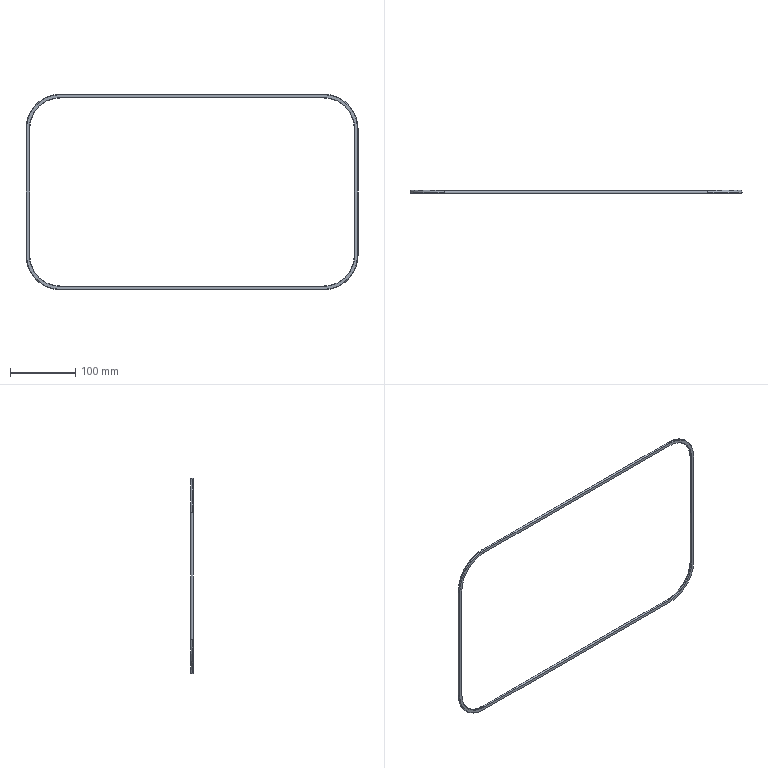Part | STEP file | P-0102091 | 1 solid | 17 faces | box 508.6 x 4.6 x 299.7 mm | volume 33274 mm3 | torus 12 | cylinder 4 | plane 1 | commonest cylinder face diameters 5.7 x4
STEP:
#1=CARTESIAN_POINT('',(0.,0.,0.));
#2=DIRECTION('',(0.,0.,1.));
#3=DIRECTION('',(1.,0.,0.));
#4=AXIS2_PLACEMENT_3D('',#1,#2,#3);
#5=CARTESIAN_POINT('',(-248.8,0.,-91.5));
#6=VERTEX_POINT('',#5);
#7=CARTESIAN_POINT('',(-248.199,-1.75,-91.5));
#8=VERTEX_POINT('',#7);
#9=CARTESIAN_POINT('',(-245.95,0.,-91.5));
#10=DIRECTION('',(0.,0.,1.));
#11=DIRECTION('',(0.,-1.,0.));
#12=AXIS2_PLACEMENT_3D('',#9,#10,#11);
#13=CIRCLE('',#12,2.85);
#14=CARTESIAN_POINT('',(-195.95,0.,-91.5));
#15=DIRECTION('',(0.,-1.,0.));
#16=DIRECTION('',(0.,0.,-1.));
#17=AXIS2_PLACEMENT_3D('',#14,#15,#16);
#18=TOROIDAL_SURFACE('',#17,50.,2.85);
#19=CARTESIAN_POINT('',(4.712,-4.712));
#20=DIRECTION('',(0.,1.));
#21=VECTOR('',#20,1.);
#22=LINE('',#19,#21);
#23=(GEOMETRIC_REPRESENTATION_CONTEXT(2)PARAMETRIC_REPRESENTATION_CONTEXT()REPRESENTATION_CONTEXT('',''));
#24=DEFINITIONAL_REPRESENTATION('',(#22),#23);
#25=PCURVE('',#18,#24);
#26=CARTESIAN_POINT('',(-245.95,0.,102.5));
#27=DIRECTION('',(0.,0.,-1.));
#28=DIRECTION('',(0.,-1.,0.));
#29=AXIS2_PLACEMENT_3D('',#26,#27,#28);
#30=CYLINDRICAL_SURFACE('',#29,2.85);
#31=CARTESIAN_POINT('',(6.283,194.));
#32=DIRECTION('',(-1.,0.));
#33=VECTOR('',#32,1.);
#34=LINE('',#31,#33);
#35=(GEOMETRIC_REPRESENTATION_CONTEXT(2)PARAMETRIC_REPRESENTATION_CONTEXT()REPRESENTATION_CONTEXT('',''));
#36=DEFINITIONAL_REPRESENTATION('',(#34),#35);
#37=PCURVE('',#30,#36);
#38=SURFACE_CURVE('',#13,(#25,#37),.PCURVE_S1.);
#39=EDGE_CURVE('',#6,#8,#38,.T.);
#40=ORIENTED_EDGE('',*,*,#39,.F.);
#41=CARTESIAN_POINT('',(-195.95,0.,-144.35));
#42=VERTEX_POINT('',#41);
#43=CARTESIAN_POINT('',(-195.95,0.,-91.5));
#44=DIRECTION('',(0.,-1.,0.));
#45=DIRECTION('',(1.,0.,0.));
#46=AXIS2_PLACEMENT_3D('',#43,#44,#45);
#47=CIRCLE('',#46,52.85);
#48=CARTESIAN_POINT('',(1.571,0.));
#49=DIRECTION('',(1.,0.));
#50=VECTOR('',#49,1.);
#51=LINE('',#48,#50);
#52=(GEOMETRIC_REPRESENTATION_CONTEXT(2)PARAMETRIC_REPRESENTATION_CONTEXT()REPRESENTATION_CONTEXT('',''));
#53=DEFINITIONAL_REPRESENTATION('',(#51),#52);
#54=PCURVE('',#18,#53);
#55=CARTESIAN_POINT('',(-195.95,0.,-91.5));
#56=DIRECTION('',(0.,-1.,0.));
#57=DIRECTION('',(0.,0.,-1.));
#58=AXIS2_PLACEMENT_3D('',#55,#56,#57);
#59=TOROIDAL_SURFACE('',#58,50.,2.85);
#60=CARTESIAN_POINT('',(1.571,6.283));
#61=DIRECTION('',(1.,0.));
#62=VECTOR('',#61,1.);
#63=LINE('',#60,#62);
#64=(GEOMETRIC_REPRESENTATION_CONTEXT(2)PARAMETRIC_REPRESENTATION_CONTEXT()REPRESENTATION_CONTEXT('',''));
#65=DEFINITIONAL_REPRESENTATION('',(#63),#64);
#66=PCURVE('',#59,#65);
#67=SURFACE_CURVE('',#47,(#54,#66),.PCURVE_S1.);
#68=EDGE_CURVE('',#6,#42,#67,.T.);
#69=ORIENTED_EDGE('',*,*,#68,.T.);
#70=CARTESIAN_POINT('',(-195.95,-1.75,-143.749));
#71=VERTEX_POINT('',#70);
#72=CARTESIAN_POINT('',(-195.95,0.,-141.5));
#73=DIRECTION('',(-1.,0.,0.));
#74=DIRECTION('',(0.,-1.,0.));
#75=AXIS2_PLACEMENT_3D('',#72,#73,#74);
#76=CIRCLE('',#75,2.85);
#77=CARTESIAN_POINT('',(6.283,-4.712));
#78=DIRECTION('',(0.,1.));
#79=VECTOR('',#78,1.);
#80=LINE('',#77,#79);
#81=(GEOMETRIC_REPRESENTATION_CONTEXT(2)PARAMETRIC_REPRESENTATION_CONTEXT()REPRESENTATION_CONTEXT('',''));
#82=DEFINITIONAL_REPRESENTATION('',(#80),#81);
#83=PCURVE('',#18,#82);
#84=CARTESIAN_POINT('',(-195.95,0.,-141.5));
#85=DIRECTION('',(1.,0.,0.));
#86=DIRECTION('',(0.,-1.,0.));
#87=AXIS2_PLACEMENT_3D('',#84,#85,#86);
#88=CYLINDRICAL_SURFACE('',#87,2.85);
#89=CARTESIAN_POINT('',(6.283,0.));
#90=DIRECTION('',(-1.,0.));
#91=VECTOR('',#90,1.);
#92=LINE('',#89,#91);
#93=(GEOMETRIC_REPRESENTATION_CONTEXT(2)PARAMETRIC_REPRESENTATION_CONTEXT()REPRESENTATION_CONTEXT('',''));
#94=DEFINITIONAL_REPRESENTATION('',(#92),#93);
#95=PCURVE('',#88,#94);
#96=SURFACE_CURVE('',#76,(#83,#95),.PCURVE_S1.);
#97=EDGE_CURVE('',#42,#71,#96,.T.);
#98=ORIENTED_EDGE('',*,*,#97,.T.);
#99=CARTESIAN_POINT('',(-195.95,-1.75,-91.5));
#100=DIRECTION('',(0.,1.,0.));
#101=DIRECTION('',(0.,0.,-1.));
#102=AXIS2_PLACEMENT_3D('',#99,#100,#101);
#103=CIRCLE('',#102,52.249);
#104=CARTESIAN_POINT('',(6.283,0.6612));
#105=DIRECTION('',(-1.,0.));
#106=VECTOR('',#105,1.);
#107=LINE('',#104,#106);
#108=(GEOMETRIC_REPRESENTATION_CONTEXT(2)PARAMETRIC_REPRESENTATION_CONTEXT()REPRESENTATION_CONTEXT('',''));
#109=DEFINITIONAL_REPRESENTATION('',(#107),#108);
#110=PCURVE('',#18,#109);
#111=CARTESIAN_POINT('',(-195.95,-1.75,158.523));
#112=DIRECTION('',(0.,1.,0.));
#113=DIRECTION('',(1.,0.,0.));
#114=AXIS2_PLACEMENT_3D('',#111,#112,#113);
#115=PLANE('',#114);
#116=CARTESIAN_POINT('',(0.,250.023));
#117=DIRECTION('',(0.,1.));
#118=AXIS2_PLACEMENT_2D('',#116,#117);
#119=CIRCLE('',#118,52.249);
#120=(GEOMETRIC_REPRESENTATION_CONTEXT(2)PARAMETRIC_REPRESENTATION_CONTEXT()REPRESENTATION_CONTEXT('',''));
#121=DEFINITIONAL_REPRESENTATION('',(#119),#120);
#122=PCURVE('',#115,#121);
#123=SURFACE_CURVE('',#103,(#110,#122),.PCURVE_S1.);
#124=EDGE_CURVE('',#71,#8,#123,.T.);
#125=ORIENTED_EDGE('',*,*,#124,.T.);
#126=EDGE_LOOP('',(#40,#69,#98,#125));
#127=FACE_BOUND('',#126,.T.);
#128=ADVANCED_FACE('',(#127),#18,.T.);
#129=ORIENTED_EDGE('',*,*,#68,.F.);
#130=CARTESIAN_POINT('',(-243.1,0.,-91.5));
#131=VERTEX_POINT('',#130);
#132=CARTESIAN_POINT('',(-245.95,0.,-91.5));
#133=DIRECTION('',(0.,0.,1.));
#134=DIRECTION('',(0.,-1.,0.));
#135=AXIS2_PLACEMENT_3D('',#132,#133,#134);
#136=CIRCLE('',#135,2.85);
#137=CARTESIAN_POINT('',(4.712,1.571));
#138=DIRECTION('',(0.,1.));
#139=VECTOR('',#138,1.);
#140=LINE('',#137,#139);
#141=(GEOMETRIC_REPRESENTATION_CONTEXT(2)PARAMETRIC_REPRESENTATION_CONTEXT()REPRESENTATION_CONTEXT('',''));
#142=DEFINITIONAL_REPRESENTATION('',(#140),#141);
#143=PCURVE('',#59,#142);
#144=CARTESIAN_POINT('',(6.283,194.));
#145=DIRECTION('',(-1.,0.));
#146=VECTOR('',#145,1.);
#147=LINE('',#144,#146);
#148=(GEOMETRIC_REPRESENTATION_CONTEXT(2)PARAMETRIC_REPRESENTATION_CONTEXT()REPRESENTATION_CONTEXT('',''));
#149=DEFINITIONAL_REPRESENTATION('',(#147),#148);
#150=PCURVE('',#30,#149);
#151=SURFACE_CURVE('',#136,(#143,#150),.PCURVE_S1.);
#152=EDGE_CURVE('',#131,#6,#151,.T.);
#153=ORIENTED_EDGE('',*,*,#152,.F.);
#154=CARTESIAN_POINT('',(-195.95,0.,-138.65));
#155=VERTEX_POINT('',#154);
#156=CARTESIAN_POINT('',(-195.95,0.,-91.5));
#157=DIRECTION('',(0.,-1.,0.));
#158=DIRECTION('',(1.,0.,0.));
#159=AXIS2_PLACEMENT_3D('',#156,#157,#158);
#160=CIRCLE('',#159,47.15);
#161=CARTESIAN_POINT('',(1.571,3.142));
#162=DIRECTION('',(1.,0.));
#163=VECTOR('',#162,1.);
#164=LINE('',#161,#163);
#165=(GEOMETRIC_REPRESENTATION_CONTEXT(2)PARAMETRIC_REPRESENTATION_CONTEXT()REPRESENTATION_CONTEXT('',''));
#166=DEFINITIONAL_REPRESENTATION('',(#164),#165);
#167=PCURVE('',#59,#166);
#168=CARTESIAN_POINT('',(-195.95,0.,-91.5));
#169=DIRECTION('',(0.,-1.,0.));
#170=DIRECTION('',(0.,0.,-1.));
#171=AXIS2_PLACEMENT_3D('',#168,#169,#170);
#172=TOROIDAL_SURFACE('',#171,50.,2.85);
#173=CARTESIAN_POINT('',(1.571,3.142));
#174=DIRECTION('',(1.,0.));
#175=VECTOR('',#174,1.);
#176=LINE('',#173,#175);
#177=(GEOMETRIC_REPRESENTATION_CONTEXT(2)PARAMETRIC_REPRESENTATION_CONTEXT()REPRESENTATION_CONTEXT('',''));
#178=DEFINITIONAL_REPRESENTATION('',(#176),#177);
#179=PCURVE('',#172,#178);
#180=SURFACE_CURVE('',#160,(#167,#179),.PCURVE_S1.);
#181=EDGE_CURVE('',#131,#155,#180,.T.);
#182=ORIENTED_EDGE('',*,*,#181,.T.);
#183=CARTESIAN_POINT('',(-195.95,0.,-141.5));
#184=DIRECTION('',(-1.,0.,0.));
#185=DIRECTION('',(0.,-1.,0.));
#186=AXIS2_PLACEMENT_3D('',#183,#184,#185);
#187=CIRCLE('',#186,2.85);
#188=CARTESIAN_POINT('',(6.283,1.571));
#189=DIRECTION('',(0.,1.));
#190=VECTOR('',#189,1.);
#191=LINE('',#188,#190);
#192=(GEOMETRIC_REPRESENTATION_CONTEXT(2)PARAMETRIC_REPRESENTATION_CONTEXT()REPRESENTATION_CONTEXT('',''));
#193=DEFINITIONAL_REPRESENTATION('',(#191),#192);
#194=PCURVE('',#59,#193);
#195=CARTESIAN_POINT('',(6.283,0.));
#196=DIRECTION('',(-1.,0.));
#197=VECTOR('',#196,1.);
#198=LINE('',#195,#197);
#199=(GEOMETRIC_REPRESENTATION_CONTEXT(2)PARAMETRIC_REPRESENTATION_CONTEXT()REPRESENTATION_CONTEXT('',''));
#200=DEFINITIONAL_REPRESENTATION('',(#198),#199);
#201=PCURVE('',#88,#200);
#202=SURFACE_CURVE('',#187,(#194,#201),.PCURVE_S1.);
#203=EDGE_CURVE('',#155,#42,#202,.T.);
#204=ORIENTED_EDGE('',*,*,#203,.T.);
#205=EDGE_LOOP('',(#129,#153,#182,#204));
#206=FACE_BOUND('',#205,.T.);
#207=ADVANCED_FACE('',(#206),#59,.T.);
#208=CARTESIAN_POINT('',(-195.95,0.,155.35));
#209=VERTEX_POINT('',#208);
#210=CARTESIAN_POINT('',(-195.95,-1.75,154.749));
#211=VERTEX_POINT('',#210);
#212=CARTESIAN_POINT('',(-195.95,0.,152.5));
#213=DIRECTION('',(1.,0.,0.));
#214=DIRECTION('',(0.,-1.,0.));
#215=AXIS2_PLACEMENT_3D('',#212,#213,#214);
#216=CIRCLE('',#215,2.85);
#217=CARTESIAN_POINT('',(-195.95,0.,102.5));
#218=DIRECTION('',(0.,-1.,0.));
#219=DIRECTION('',(0.,0.,-1.));
#220=AXIS2_PLACEMENT_3D('',#217,#218,#219);
#221=TOROIDAL_SURFACE('',#220,50.,2.85);
#222=CARTESIAN_POINT('',(3.142,-4.712));
#223=DIRECTION('',(0.,1.));
#224=VECTOR('',#223,1.);
#225=LINE('',#222,#224);
#226=(GEOMETRIC_REPRESENTATION_CONTEXT(2)PARAMETRIC_REPRESENTATION_CONTEXT()REPRESENTATION_CONTEXT('',''));
#227=DEFINITIONAL_REPRESENTATION('',(#225),#226);
#228=PCURVE('',#221,#227);
#229=CARTESIAN_POINT('',(206.95,0.,152.5));
#230=DIRECTION('',(-1.,0.,0.));
#231=DIRECTION('',(0.,-1.,0.));
#232=AXIS2_PLACEMENT_3D('',#229,#230,#231);
#233=CYLINDRICAL_SURFACE('',#232,2.85);
#234=CARTESIAN_POINT('',(6.283,402.9));
#235=DIRECTION('',(-1.,0.));
#236=VECTOR('',#235,1.);
#237=LINE('',#234,#236);
#238=(GEOMETRIC_REPRESENTATION_CONTEXT(2)PARAMETRIC_REPRESENTATION_CONTEXT()REPRESENTATION_CONTEXT('',''));
#239=DEFINITIONAL_REPRESENTATION('',(#237),#238);
#240=PCURVE('',#233,#239);
#241=SURFACE_CURVE('',#216,(#228,#240),.PCURVE_S1.);
#242=EDGE_CURVE('',#209,#211,#241,.T.);
#243=ORIENTED_EDGE('',*,*,#242,.F.);
#244=CARTESIAN_POINT('',(-248.8,0.,102.5));
#245=VERTEX_POINT('',#244);
#246=CARTESIAN_POINT('',(-195.95,0.,102.5));
#247=DIRECTION('',(0.,-1.,0.));
#248=DIRECTION('',(1.,0.,0.));
#249=AXIS2_PLACEMENT_3D('',#246,#247,#248);
#250=CIRCLE('',#249,52.85);
#251=CARTESIAN_POINT('',(1.571,0.));
#252=DIRECTION('',(1.,0.));
#253=VECTOR('',#252,1.);
#254=LINE('',#251,#253);
#255=(GEOMETRIC_REPRESENTATION_CONTEXT(2)PARAMETRIC_REPRESENTATION_CONTEXT()REPRESENTATION_CONTEXT('',''));
#256=DEFINITIONAL_REPRESENTATION('',(#254),#255);
#257=PCURVE('',#221,#256);
#258=CARTESIAN_POINT('',(-195.95,0.,102.5));
#259=DIRECTION('',(0.,-1.,0.));
#260=DIRECTION('',(0.,0.,-1.));
#261=AXIS2_PLACEMENT_3D('',#258,#259,#260);
#262=TOROIDAL_SURFACE('',#261,50.,2.85);
#263=CARTESIAN_POINT('',(1.571,6.283));
#264=DIRECTION('',(1.,0.));
#265=VECTOR('',#264,1.);
#266=LINE('',#263,#265);
#267=(GEOMETRIC_REPRESENTATION_CONTEXT(2)PARAMETRIC_REPRESENTATION_CONTEXT()REPRESENTATION_CONTEXT('',''));
#268=DEFINITIONAL_REPRESENTATION('',(#266),#267);
#269=PCURVE('',#262,#268);
#270=SURFACE_CURVE('',#250,(#257,#269),.PCURVE_S1.);
#271=EDGE_CURVE('',#209,#245,#270,.T.);
#272=ORIENTED_EDGE('',*,*,#271,.T.);
#273=CARTESIAN_POINT('',(-248.199,-1.75,102.5));
#274=VERTEX_POINT('',#273);
#275=CARTESIAN_POINT('',(-245.95,0.,102.5));
#276=DIRECTION('',(0.,0.,1.));
#277=DIRECTION('',(0.,-1.,0.));
#278=AXIS2_PLACEMENT_3D('',#275,#276,#277);
#279=CIRCLE('',#278,2.85);
#280=CARTESIAN_POINT('',(4.712,-4.712));
#281=DIRECTION('',(0.,1.));
#282=VECTOR('',#281,1.);
#283=LINE('',#280,#282);
#284=(GEOMETRIC_REPRESENTATION_CONTEXT(2)PARAMETRIC_REPRESENTATION_CONTEXT()REPRESENTATION_CONTEXT('',''));
#285=DEFINITIONAL_REPRESENTATION('',(#283),#284);
#286=PCURVE('',#221,#285);
#287=CARTESIAN_POINT('',(6.283,0.));
#288=DIRECTION('',(-1.,0.));
#289=VECTOR('',#288,1.);
#290=LINE('',#287,#289);
#291=(GEOMETRIC_REPRESENTATION_CONTEXT(2)PARAMETRIC_REPRESENTATION_CONTEXT()REPRESENTATION_CONTEXT('',''));
#292=DEFINITIONAL_REPRESENTATION('',(#290),#291);
#293=PCURVE('',#30,#292);
#294=SURFACE_CURVE('',#279,(#286,#293),.PCURVE_S1.);
#295=EDGE_CURVE('',#245,#274,#294,.T.);
#296=ORIENTED_EDGE('',*,*,#295,.T.);
#297=CARTESIAN_POINT('',(-195.95,-1.75,102.5));
#298=DIRECTION('',(0.,1.,0.));
#299=DIRECTION('',(0.,0.,-1.));
#300=AXIS2_PLACEMENT_3D('',#297,#298,#299);
#301=CIRCLE('',#300,52.249);
#302=CARTESIAN_POINT('',(6.283,0.6612));
#303=DIRECTION('',(-1.,0.));
#304=VECTOR('',#303,1.);
#305=LINE('',#302,#304);
#306=(GEOMETRIC_REPRESENTATION_CONTEXT(2)PARAMETRIC_REPRESENTATION_CONTEXT()REPRESENTATION_CONTEXT('',''));
#307=DEFINITIONAL_REPRESENTATION('',(#305),#306);
#308=PCURVE('',#221,#307);
#309=CARTESIAN_POINT('',(0.,56.023));
#310=DIRECTION('',(0.,1.));
#311=AXIS2_PLACEMENT_2D('',#309,#310);
#312=CIRCLE('',#311,52.249);
#313=(GEOMETRIC_REPRESENTATION_CONTEXT(2)PARAMETRIC_REPRESENTATION_CONTEXT()REPRESENTATION_CONTEXT('',''));
#314=DEFINITIONAL_REPRESENTATION('',(#312),#313);
#315=PCURVE('',#115,#314);
#316=SURFACE_CURVE('',#301,(#308,#315),.PCURVE_S1.);
#317=EDGE_CURVE('',#274,#211,#316,.T.);
#318=ORIENTED_EDGE('',*,*,#317,.T.);
#319=EDGE_LOOP('',(#243,#272,#296,#318));
#320=FACE_BOUND('',#319,.T.);
#321=ADVANCED_FACE('',(#320),#221,.T.);
#322=ORIENTED_EDGE('',*,*,#271,.F.);
#323=CARTESIAN_POINT('',(-195.95,0.,149.65));
#324=VERTEX_POINT('',#323);
#325=CARTESIAN_POINT('',(-195.95,0.,152.5));
#326=DIRECTION('',(1.,0.,0.));
#327=DIRECTION('',(0.,-1.,0.));
#328=AXIS2_PLACEMENT_3D('',#325,#326,#327);
#329=CIRCLE('',#328,2.85);
#330=CARTESIAN_POINT('',(3.142,1.571));
#331=DIRECTION('',(0.,1.));
#332=VECTOR('',#331,1.);
#333=LINE('',#330,#332);
#334=(GEOMETRIC_REPRESENTATION_CONTEXT(2)PARAMETRIC_REPRESENTATION_CONTEXT()REPRESENTATION_CONTEXT('',''));
#335=DEFINITIONAL_REPRESENTATION('',(#333),#334);
#336=PCURVE('',#262,#335);
#337=CARTESIAN_POINT('',(6.283,402.9));
#338=DIRECTION('',(-1.,0.));
#339=VECTOR('',#338,1.);
#340=LINE('',#337,#339);
#341=(GEOMETRIC_REPRESENTATION_CONTEXT(2)PARAMETRIC_REPRESENTATION_CONTEXT()REPRESENTATION_CONTEXT('',''));
#342=DEFINITIONAL_REPRESENTATION('',(#340),#341);
#343=PCURVE('',#233,#342);
#344=SURFACE_CURVE('',#329,(#336,#343),.PCURVE_S1.);
#345=EDGE_CURVE('',#324,#209,#344,.T.);
#346=ORIENTED_EDGE('',*,*,#345,.F.);
#347=CARTESIAN_POINT('',(-243.1,0.,102.5));
#348=VERTEX_POINT('',#347);
#349=CARTESIAN_POINT('',(-195.95,0.,102.5));
#350=DIRECTION('',(0.,-1.,0.));
#351=DIRECTION('',(1.,0.,0.));
#352=AXIS2_PLACEMENT_3D('',#349,#350,#351);
#353=CIRCLE('',#352,47.15);
#354=CARTESIAN_POINT('',(1.571,3.142));
#355=DIRECTION('',(1.,0.));
#356=VECTOR('',#355,1.);
#357=LINE('',#354,#356);
#358=(GEOMETRIC_REPRESENTATION_CONTEXT(2)PARAMETRIC_REPRESENTATION_CONTEXT()REPRESENTATION_CONTEXT('',''));
#359=DEFINITIONAL_REPRESENTATION('',(#357),#358);
#360=PCURVE('',#262,#359);
#361=CARTESIAN_POINT('',(-195.95,0.,102.5));
#362=DIRECTION('',(0.,-1.,0.));
#363=DIRECTION('',(0.,0.,-1.));
#364=AXIS2_PLACEMENT_3D('',#361,#362,#363);
#365=TOROIDAL_SURFACE('',#364,50.,2.85);
#366=CARTESIAN_POINT('',(1.571,3.142));
#367=DIRECTION('',(1.,0.));
#368=VECTOR('',#367,1.);
#369=LINE('',#366,#368);
#370=(GEOMETRIC_REPRESENTATION_CONTEXT(2)PARAMETRIC_REPRESENTATION_CONTEXT()REPRESENTATION_CONTEXT('',''));
#371=DEFINITIONAL_REPRESENTATION('',(#369),#370);
#372=PCURVE('',#365,#371);
#373=SURFACE_CURVE('',#353,(#360,#372),.PCURVE_S1.);
#374=EDGE_CURVE('',#324,#348,#373,.T.);
#375=ORIENTED_EDGE('',*,*,#374,.T.);
#376=CARTESIAN_POINT('',(-245.95,0.,102.5));
#377=DIRECTION('',(0.,0.,1.));
#378=DIRECTION('',(0.,-1.,0.));
#379=AXIS2_PLACEMENT_3D('',#376,#377,#378);
#380=CIRCLE('',#379,2.85);
#381=CARTESIAN_POINT('',(4.712,1.571));
#382=DIRECTION('',(0.,1.));
#383=VECTOR('',#382,1.);
#384=LINE('',#381,#383);
#385=(GEOMETRIC_REPRESENTATION_CONTEXT(2)PARAMETRIC_REPRESENTATION_CONTEXT()REPRESENTATION_CONTEXT('',''));
#386=DEFINITIONAL_REPRESENTATION('',(#384),#385);
#387=PCURVE('',#262,#386);
#388=CARTESIAN_POINT('',(6.283,0.));
#389=DIRECTION('',(-1.,0.));
#390=VECTOR('',#389,1.);
#391=LINE('',#388,#390);
#392=(GEOMETRIC_REPRESENTATION_CONTEXT(2)PARAMETRIC_REPRESENTATION_CONTEXT()REPRESENTATION_CONTEXT('',''));
#393=DEFINITIONAL_REPRESENTATION('',(#391),#392);
#394=PCURVE('',#30,#393);
#395=SURFACE_CURVE('',#380,(#387,#394),.PCURVE_S1.);
#396=EDGE_CURVE('',#348,#245,#395,.T.);
#397=ORIENTED_EDGE('',*,*,#396,.T.);
#398=EDGE_LOOP('',(#322,#346,#375,#397));
#399=FACE_BOUND('',#398,.T.);
#400=ADVANCED_FACE('',(#399),#262,.T.);
#401=CARTESIAN_POINT('',(259.8,0.,102.5));
#402=VERTEX_POINT('',#401);
#403=CARTESIAN_POINT('',(259.199,-1.75,102.5));
#404=VERTEX_POINT('',#403);
#405=CARTESIAN_POINT('',(256.95,0.,102.5));
#406=DIRECTION('',(0.,0.,-1.));
#407=DIRECTION('',(0.,-1.,0.));
#408=AXIS2_PLACEMENT_3D('',#405,#406,#407);
#409=CIRCLE('',#408,2.85);
#410=CARTESIAN_POINT('',(206.95,0.,102.5));
#411=DIRECTION('',(0.,-1.,0.));
#412=DIRECTION('',(0.,0.,-1.));
#413=AXIS2_PLACEMENT_3D('',#410,#411,#412);
#414=TOROIDAL_SURFACE('',#413,50.,2.85);
#415=CARTESIAN_POINT('',(1.571,-4.712));
#416=DIRECTION('',(0.,1.));
#417=VECTOR('',#416,1.);
#418=LINE('',#415,#417);
#419=(GEOMETRIC_REPRESENTATION_CONTEXT(2)PARAMETRIC_REPRESENTATION_CONTEXT()REPRESENTATION_CONTEXT('',''));
#420=DEFINITIONAL_REPRESENTATION('',(#418),#419);
#421=PCURVE('',#414,#420);
#422=CARTESIAN_POINT('',(256.95,0.,-91.5));
#423=DIRECTION('',(0.,0.,1.));
#424=DIRECTION('',(0.,-1.,0.));
#425=AXIS2_PLACEMENT_3D('',#422,#423,#424);
#426=CYLINDRICAL_SURFACE('',#425,2.85);
#427=CARTESIAN_POINT('',(6.283,194.));
#428=DIRECTION('',(-1.,0.));
#429=VECTOR('',#428,1.);
#430=LINE('',#427,#429);
#431=(GEOMETRIC_REPRESENTATION_CONTEXT(2)PARAMETRIC_REPRESENTATION_CONTEXT()REPRESENTATION_CONTEXT('',''));
#432=DEFINITIONAL_REPRESENTATION('',(#430),#431);
#433=PCURVE('',#426,#432);
#434=SURFACE_CURVE('',#409,(#421,#433),.PCURVE_S1.);
#435=EDGE_CURVE('',#402,#404,#434,.T.);
#436=ORIENTED_EDGE('',*,*,#435,.F.);
#437=CARTESIAN_POINT('',(206.95,0.,155.35));
#438=VERTEX_POINT('',#437);
#439=CARTESIAN_POINT('',(206.95,0.,102.5));
#440=DIRECTION('',(0.,-1.,0.));
#441=DIRECTION('',(1.,0.,0.));
#442=AXIS2_PLACEMENT_3D('',#439,#440,#441);
#443=CIRCLE('',#442,52.85);
#444=CARTESIAN_POINT('',(1.571,0.));
#445=DIRECTION('',(1.,0.));
#446=VECTOR('',#445,1.);
#447=LINE('',#444,#446);
#448=(GEOMETRIC_REPRESENTATION_CONTEXT(2)PARAMETRIC_REPRESENTATION_CONTEXT()REPRESENTATION_CONTEXT('',''));
#449=DEFINITIONAL_REPRESENTATION('',(#447),#448);
#450=PCURVE('',#414,#449);
#451=CARTESIAN_POINT('',(206.95,0.,102.5));
#452=DIRECTION('',(0.,-1.,0.));
#453=DIRECTION('',(0.,0.,-1.));
#454=AXIS2_PLACEMENT_3D('',#451,#452,#453);
#455=TOROIDAL_SURFACE('',#454,50.,2.85);
#456=CARTESIAN_POINT('',(1.571,6.283));
#457=CARTESIAN_POINT('',(1.595,6.283));
#458=CARTESIAN_POINT('',(1.642,6.283));
#459=CARTESIAN_POINT('',(1.714,6.283));
#460=CARTESIAN_POINT('',(1.785,6.283));
#461=CARTESIAN_POINT('',(1.856,6.283));
#462=CARTESIAN_POINT('',(1.928,6.283));
#463=CARTESIAN_POINT('',(1.999,6.283));
#464=CARTESIAN_POINT('',(2.071,6.283));
#465=CARTESIAN_POINT('',(2.142,6.283));
#466=CARTESIAN_POINT('',(2.213,6.283));
#467=CARTESIAN_POINT('',(2.285,6.283));
#468=CARTESIAN_POINT('',(2.356,6.283));
#469=CARTESIAN_POINT('',(2.428,6.283));
#470=CARTESIAN_POINT('',(2.499,6.283));
#471=CARTESIAN_POINT('',(2.57,6.283));
#472=CARTESIAN_POINT('',(2.642,6.283));
#473=CARTESIAN_POINT('',(2.713,6.283));
#474=CARTESIAN_POINT('',(2.785,6.283));
#475=CARTESIAN_POINT('',(2.856,6.283));
#476=CARTESIAN_POINT('',(2.927,6.283));
#477=CARTESIAN_POINT('',(2.999,6.283));
#478=CARTESIAN_POINT('',(3.07,6.283));
#479=CARTESIAN_POINT('',(3.118,6.283));
#480=CARTESIAN_POINT('',(3.142,6.283));
#481=B_SPLINE_CURVE_WITH_KNOTS('',3,(#456,#457,#458,#459,#460,#461,#462,#463,#464,#465,#466,#467,#468,#469,#470,#471,#472,#473,#474,#475,#476,#477,#478,#479,#480),.UNSPECIFIED.,.F.,.F.,(4,1,1,1,1,1,1,1,1,1,1,1,1,1,1,1,1,1,1,1,1,1,4),(0.,0.0714,0.1428,0.2142,0.2856,0.357,0.4284,0.4998,0.5712,0.6426,0.714,0.7854,0.8568,0.9282,0.9996,1.071,1.142,1.214,1.285,1.357,1.428,1.499,1.571),.QUASI_UNIFORM_KNOTS.);
#482=(GEOMETRIC_REPRESENTATION_CONTEXT(2)PARAMETRIC_REPRESENTATION_CONTEXT()REPRESENTATION_CONTEXT('',''));
#483=DEFINITIONAL_REPRESENTATION('',(#481),#482);
#484=PCURVE('',#455,#483);
#485=SURFACE_CURVE('',#443,(#450,#484),.PCURVE_S1.);
#486=EDGE_CURVE('',#402,#438,#485,.T.);
#487=ORIENTED_EDGE('',*,*,#486,.T.);
#488=CARTESIAN_POINT('',(206.95,-1.75,154.749));
#489=VERTEX_POINT('',#488);
#490=CARTESIAN_POINT('',(206.95,0.,152.5));
#491=DIRECTION('',(1.,0.,0.));
#492=DIRECTION('',(0.,-1.,0.));
#493=AXIS2_PLACEMENT_3D('',#490,#491,#492);
#494=CIRCLE('',#493,2.85);
#495=CARTESIAN_POINT('',(3.142,-4.712));
#496=DIRECTION('',(0.,1.));
#497=VECTOR('',#496,1.);
#498=LINE('',#495,#497);
#499=(GEOMETRIC_REPRESENTATION_CONTEXT(2)PARAMETRIC_REPRESENTATION_CONTEXT()REPRESENTATION_CONTEXT('',''));
#500=DEFINITIONAL_REPRESENTATION('',(#498),#499);
#501=PCURVE('',#414,#500);
#502=CARTESIAN_POINT('',(6.283,0.));
#503=DIRECTION('',(-1.,0.));
#504=VECTOR('',#503,1.);
#505=LINE('',#502,#504);
#506=(GEOMETRIC_REPRESENTATION_CONTEXT(2)PARAMETRIC_REPRESENTATION_CONTEXT()REPRESENTATION_CONTEXT('',''));
#507=DEFINITIONAL_REPRESENTATION('',(#505),#506);
#508=PCURVE('',#233,#507);
#509=SURFACE_CURVE('',#494,(#501,#508),.PCURVE_S1.);
#510=EDGE_CURVE('',#438,#489,#509,.T.);
#511=ORIENTED_EDGE('',*,*,#510,.T.);
#512=CARTESIAN_POINT('',(206.95,-1.75,102.5));
#513=DIRECTION('',(0.,1.,0.));
#514=DIRECTION('',(0.,0.,-1.));
#515=AXIS2_PLACEMENT_3D('',#512,#513,#514);
#516=CIRCLE('',#515,52.249);
#517=CARTESIAN_POINT('',(6.283,0.6612));
#518=DIRECTION('',(-1.,0.));
#519=VECTOR('',#518,1.);
#520=LINE('',#517,#519);
#521=(GEOMETRIC_REPRESENTATION_CONTEXT(2)PARAMETRIC_REPRESENTATION_CONTEXT()REPRESENTATION_CONTEXT('',''));
#522=DEFINITIONAL_REPRESENTATION('',(#520),#521);
#523=PCURVE('',#414,#522);
#524=CARTESIAN_POINT('',(402.9,56.023));
#525=DIRECTION('',(0.,1.));
#526=AXIS2_PLACEMENT_2D('',#524,#525);
#527=CIRCLE('',#526,52.249);
#528=(GEOMETRIC_REPRESENTATION_CONTEXT(2)PARAMETRIC_REPRESENTATION_CONTEXT()REPRESENTATION_CONTEXT('',''));
#529=DEFINITIONAL_REPRESENTATION('',(#527),#528);
#530=PCURVE('',#115,#529);
#531=SURFACE_CURVE('',#516,(#523,#530),.PCURVE_S1.);
#532=EDGE_CURVE('',#489,#404,#531,.T.);
#533=ORIENTED_EDGE('',*,*,#532,.T.);
#534=EDGE_LOOP('',(#436,#487,#511,#533));
#535=FACE_BOUND('',#534,.T.);
#536=ADVANCED_FACE('',(#535),#414,.T.);
#537=ORIENTED_EDGE('',*,*,#486,.F.);
#538=CARTESIAN_POINT('',(254.1,0.,102.5));
#539=VERTEX_POINT('',#538);
#540=CARTESIAN_POINT('',(256.95,0.,102.5));
#541=DIRECTION('',(0.,0.,-1.));
#542=DIRECTION('',(0.,-1.,0.));
#543=AXIS2_PLACEMENT_3D('',#540,#541,#542);
#544=CIRCLE('',#543,2.85);
#545=CARTESIAN_POINT('',(1.571,1.571));
#546=DIRECTION('',(0.,1.));
#547=VECTOR('',#546,1.);
#548=LINE('',#545,#547);
#549=(GEOMETRIC_REPRESENTATION_CONTEXT(2)PARAMETRIC_REPRESENTATION_CONTEXT()REPRESENTATION_CONTEXT('',''));
#550=DEFINITIONAL_REPRESENTATION('',(#548),#549);
#551=PCURVE('',#455,#550);
#552=CARTESIAN_POINT('',(6.283,194.));
#553=DIRECTION('',(-1.,0.));
#554=VECTOR('',#553,1.);
#555=LINE('',#552,#554);
#556=(GEOMETRIC_REPRESENTATION_CONTEXT(2)PARAMETRIC_REPRESENTATION_CONTEXT()REPRESENTATION_CONTEXT('',''));
#557=DEFINITIONAL_REPRESENTATION('',(#555),#556);
#558=PCURVE('',#426,#557);
#559=SURFACE_CURVE('',#544,(#551,#558),.PCURVE_S1.);
#560=EDGE_CURVE('',#539,#402,#559,.T.);
#561=ORIENTED_EDGE('',*,*,#560,.F.);
#562=CARTESIAN_POINT('',(206.95,0.,149.65));
#563=VERTEX_POINT('',#562);
#564=CARTESIAN_POINT('',(206.95,0.,102.5));
#565=DIRECTION('',(0.,-1.,0.));
#566=DIRECTION('',(1.,0.,0.));
#567=AXIS2_PLACEMENT_3D('',#564,#565,#566);
#568=CIRCLE('',#567,47.15);
#569=CARTESIAN_POINT('',(1.571,3.142));
#570=DIRECTION('',(1.,0.));
#571=VECTOR('',#570,1.);
#572=LINE('',#569,#571);
#573=(GEOMETRIC_REPRESENTATION_CONTEXT(2)PARAMETRIC_REPRESENTATION_CONTEXT()REPRESENTATION_CONTEXT('',''));
#574=DEFINITIONAL_REPRESENTATION('',(#572),#573);
#575=PCURVE('',#455,#574);
#576=CARTESIAN_POINT('',(206.95,0.,102.5));
#577=DIRECTION('',(0.,-1.,0.));
#578=DIRECTION('',(0.,0.,-1.));
#579=AXIS2_PLACEMENT_3D('',#576,#577,#578);
#580=TOROIDAL_SURFACE('',#579,50.,2.85);
#581=CARTESIAN_POINT('',(1.571,3.142));
#582=DIRECTION('',(1.,0.));
#583=VECTOR('',#582,1.);
#584=LINE('',#581,#583);
#585=(GEOMETRIC_REPRESENTATION_CONTEXT(2)PARAMETRIC_REPRESENTATION_CONTEXT()REPRESENTATION_CONTEXT('',''));
#586=DEFINITIONAL_REPRESENTATION('',(#584),#585);
#587=PCURVE('',#580,#586);
#588=SURFACE_CURVE('',#568,(#575,#587),.PCURVE_S1.);
#589=EDGE_CURVE('',#539,#563,#588,.T.);
#590=ORIENTED_EDGE('',*,*,#589,.T.);
#591=CARTESIAN_POINT('',(206.95,0.,152.5));
#592=DIRECTION('',(1.,0.,0.));
#593=DIRECTION('',(0.,-1.,0.));
#594=AXIS2_PLACEMENT_3D('',#591,#592,#593);
#595=CIRCLE('',#594,2.85);
#596=CARTESIAN_POINT('',(3.142,1.571));
#597=DIRECTION('',(0.,1.));
#598=VECTOR('',#597,1.);
#599=LINE('',#596,#598);
#600=(GEOMETRIC_REPRESENTATION_CONTEXT(2)PARAMETRIC_REPRESENTATION_CONTEXT()REPRESENTATION_CONTEXT('',''));
#601=DEFINITIONAL_REPRESENTATION('',(#599),#600);
#602=PCURVE('',#455,#601);
#603=CARTESIAN_POINT('',(6.283,0.));
#604=DIRECTION('',(-1.,0.));
#605=VECTOR('',#604,1.);
#606=LINE('',#603,#605);
#607=(GEOMETRIC_REPRESENTATION_CONTEXT(2)PARAMETRIC_REPRESENTATION_CONTEXT()REPRESENTATION_CONTEXT('',''));
#608=DEFINITIONAL_REPRESENTATION('',(#606),#607);
#609=PCURVE('',#233,#608);
#610=SURFACE_CURVE('',#595,(#602,#609),.PCURVE_S1.);
#611=EDGE_CURVE('',#563,#438,#610,.T.);
#612=ORIENTED_EDGE('',*,*,#611,.T.);
#613=EDGE_LOOP('',(#537,#561,#590,#612));
#614=FACE_BOUND('',#613,.T.);
#615=ADVANCED_FACE('',(#614),#455,.T.);
#616=CARTESIAN_POINT('',(206.95,0.,-144.35));
#617=VERTEX_POINT('',#616);
#618=CARTESIAN_POINT('',(206.95,-1.75,-143.749));
#619=VERTEX_POINT('',#618);
#620=CARTESIAN_POINT('',(206.95,0.,-141.5));
#621=DIRECTION('',(-1.,0.,0.));
#622=DIRECTION('',(0.,-1.,0.));
#623=AXIS2_PLACEMENT_3D('',#620,#621,#622);
#624=CIRCLE('',#623,2.85);
#625=CARTESIAN_POINT('',(206.95,0.,-91.5));
#626=DIRECTION('',(0.,-1.,0.));
#627=DIRECTION('',(0.,0.,-1.));
#628=AXIS2_PLACEMENT_3D('',#625,#626,#627);
#629=TOROIDAL_SURFACE('',#628,50.,2.85);
#630=CARTESIAN_POINT('',(0.,-4.712));
#631=DIRECTION('',(0.,1.));
#632=VECTOR('',#631,1.);
#633=LINE('',#630,#632);
#634=(GEOMETRIC_REPRESENTATION_CONTEXT(2)PARAMETRIC_REPRESENTATION_CONTEXT()REPRESENTATION_CONTEXT('',''));
#635=DEFINITIONAL_REPRESENTATION('',(#633),#634);
#636=PCURVE('',#629,#635);
#637=CARTESIAN_POINT('',(6.283,402.9));
#638=DIRECTION('',(-1.,0.));
#639=VECTOR('',#638,1.);
#640=LINE('',#637,#639);
#641=(GEOMETRIC_REPRESENTATION_CONTEXT(2)PARAMETRIC_REPRESENTATION_CONTEXT()REPRESENTATION_CONTEXT('',''));
#642=DEFINITIONAL_REPRESENTATION('',(#640),#641);
#643=PCURVE('',#88,#642);
#644=SURFACE_CURVE('',#624,(#636,#643),.PCURVE_S1.);
#645=EDGE_CURVE('',#617,#619,#644,.T.);
#646=ORIENTED_EDGE('',*,*,#645,.F.);
#647=CARTESIAN_POINT('',(259.8,0.,-91.5));
#648=VERTEX_POINT('',#647);
#649=CARTESIAN_POINT('',(206.95,0.,-91.5));
#650=DIRECTION('',(0.,-1.,0.));
#651=DIRECTION('',(1.,0.,0.));
#652=AXIS2_PLACEMENT_3D('',#649,#650,#651);
#653=CIRCLE('',#652,52.85);
#654=CARTESIAN_POINT('',(-4.712,0.));
#655=DIRECTION('',(1.,0.));
#656=VECTOR('',#655,1.);
#657=LINE('',#654,#656);
#658=(GEOMETRIC_REPRESENTATION_CONTEXT(2)PARAMETRIC_REPRESENTATION_CONTEXT()REPRESENTATION_CONTEXT('',''));
#659=DEFINITIONAL_REPRESENTATION('',(#657),#658);
#660=PCURVE('',#629,#659);
#661=CARTESIAN_POINT('',(206.95,0.,-91.5));
#662=DIRECTION('',(0.,-1.,0.));
#663=DIRECTION('',(0.,0.,-1.));
#664=AXIS2_PLACEMENT_3D('',#661,#662,#663);
#665=TOROIDAL_SURFACE('',#664,50.,2.85);
#666=CARTESIAN_POINT('',(0.,6.283));
#667=CARTESIAN_POINT('',(0.0238,6.283));
#668=CARTESIAN_POINT('',(0.0714,6.283));
#669=CARTESIAN_POINT('',(0.1428,6.283));
#670=CARTESIAN_POINT('',(0.2142,6.283));
#671=CARTESIAN_POINT('',(0.2856,6.283));
#672=CARTESIAN_POINT('',(0.357,6.283));
#673=CARTESIAN_POINT('',(0.4284,6.283));
#674=CARTESIAN_POINT('',(0.4998,6.283));
#675=CARTESIAN_POINT('',(0.5712,6.283));
#676=CARTESIAN_POINT('',(0.6426,6.283));
#677=CARTESIAN_POINT('',(0.714,6.283));
#678=CARTESIAN_POINT('',(0.7854,6.283));
#679=CARTESIAN_POINT('',(0.8568,6.283));
#680=CARTESIAN_POINT('',(0.9282,6.283));
#681=CARTESIAN_POINT('',(0.9996,6.283));
#682=CARTESIAN_POINT('',(1.071,6.283));
#683=CARTESIAN_POINT('',(1.142,6.283));
#684=CARTESIAN_POINT('',(1.214,6.283));
#685=CARTESIAN_POINT('',(1.285,6.283));
#686=CARTESIAN_POINT('',(1.357,6.283));
#687=CARTESIAN_POINT('',(1.428,6.283));
#688=CARTESIAN_POINT('',(1.499,6.283));
#689=CARTESIAN_POINT('',(1.547,6.283));
#690=CARTESIAN_POINT('',(1.571,6.283));
#691=B_SPLINE_CURVE_WITH_KNOTS('',3,(#666,#667,#668,#669,#670,#671,#672,#673,#674,#675,#676,#677,#678,#679,#680,#681,#682,#683,#684,#685,#686,#687,#688,#689,#690),.UNSPECIFIED.,.F.,.F.,(4,1,1,1,1,1,1,1,1,1,1,1,1,1,1,1,1,1,1,1,1,1,4),(4.712,4.784,4.855,4.927,4.998,5.069,5.141,5.212,5.284,5.355,5.426,5.498,5.569,5.641,5.712,5.783,5.855,5.926,5.998,6.069,6.14,6.212,6.283),.QUASI_UNIFORM_KNOTS.);
#692=(GEOMETRIC_REPRESENTATION_CONTEXT(2)PARAMETRIC_REPRESENTATION_CONTEXT()REPRESENTATION_CONTEXT('',''));
#693=DEFINITIONAL_REPRESENTATION('',(#691),#692);
#694=PCURVE('',#665,#693);
#695=SURFACE_CURVE('',#653,(#660,#694),.PCURVE_S1.);
#696=EDGE_CURVE('',#617,#648,#695,.T.);
#697=ORIENTED_EDGE('',*,*,#696,.T.);
#698=CARTESIAN_POINT('',(259.199,-1.75,-91.5));
#699=VERTEX_POINT('',#698);
#700=CARTESIAN_POINT('',(256.95,0.,-91.5));
#701=DIRECTION('',(0.,0.,-1.));
#702=DIRECTION('',(0.,-1.,0.));
#703=AXIS2_PLACEMENT_3D('',#700,#701,#702);
#704=CIRCLE('',#703,2.85);
#705=CARTESIAN_POINT('',(1.571,-4.712));
#706=DIRECTION('',(0.,1.));
#707=VECTOR('',#706,1.);
#708=LINE('',#705,#707);
#709=(GEOMETRIC_REPRESENTATION_CONTEXT(2)PARAMETRIC_REPRESENTATION_CONTEXT()REPRESENTATION_CONTEXT('',''));
#710=DEFINITIONAL_REPRESENTATION('',(#708),#709);
#711=PCURVE('',#629,#710);
#712=CARTESIAN_POINT('',(6.283,0.));
#713=DIRECTION('',(-1.,0.));
#714=VECTOR('',#713,1.);
#715=LINE('',#712,#714);
#716=(GEOMETRIC_REPRESENTATION_CONTEXT(2)PARAMETRIC_REPRESENTATION_CONTEXT()REPRESENTATION_CONTEXT('',''));
#717=DEFINITIONAL_REPRESENTATION('',(#715),#716);
#718=PCURVE('',#426,#717);
#719=SURFACE_CURVE('',#704,(#711,#718),.PCURVE_S1.);
#720=EDGE_CURVE('',#648,#699,#719,.T.);
#721=ORIENTED_EDGE('',*,*,#720,.T.);
#722=CARTESIAN_POINT('',(206.95,-1.75,-91.5));
#723=DIRECTION('',(0.,1.,0.));
#724=DIRECTION('',(0.,0.,-1.));
#725=AXIS2_PLACEMENT_3D('',#722,#723,#724);
#726=CIRCLE('',#725,52.249);
#727=CARTESIAN_POINT('',(6.283,0.6612));
#728=DIRECTION('',(-1.,0.));
#729=VECTOR('',#728,1.);
#730=LINE('',#727,#729);
#731=(GEOMETRIC_REPRESENTATION_CONTEXT(2)PARAMETRIC_REPRESENTATION_CONTEXT()REPRESENTATION_CONTEXT('',''));
#732=DEFINITIONAL_REPRESENTATION('',(#730),#731);
#733=PCURVE('',#629,#732);
#734=CARTESIAN_POINT('',(402.9,250.023));
#735=DIRECTION('',(0.,1.));
#736=AXIS2_PLACEMENT_2D('',#734,#735);
#737=CIRCLE('',#736,52.249);
#738=(GEOMETRIC_REPRESENTATION_CONTEXT(2)PARAMETRIC_REPRESENTATION_CONTEXT()REPRESENTATION_CONTEXT('',''));
#739=DEFINITIONAL_REPRESENTATION('',(#737),#738);
#740=PCURVE('',#115,#739);
#741=SURFACE_CURVE('',#726,(#733,#740),.PCURVE_S1.);
#742=EDGE_CURVE('',#699,#619,#741,.T.);
#743=ORIENTED_EDGE('',*,*,#742,.T.);
#744=EDGE_LOOP('',(#646,#697,#721,#743));
#745=FACE_BOUND('',#744,.T.);
#746=ADVANCED_FACE('',(#745),#629,.T.);
#747=ORIENTED_EDGE('',*,*,#696,.F.);
#748=CARTESIAN_POINT('',(206.95,0.,-138.65));
#749=VERTEX_POINT('',#748);
#750=CARTESIAN_POINT('',(206.95,0.,-141.5));
#751=DIRECTION('',(-1.,0.,0.));
#752=DIRECTION('',(0.,-1.,0.));
#753=AXIS2_PLACEMENT_3D('',#750,#751,#752);
#754=CIRCLE('',#753,2.85);
#755=CARTESIAN_POINT('',(0.,1.571));
#756=DIRECTION('',(0.,1.));
#757=VECTOR('',#756,1.);
#758=LINE('',#755,#757);
#759=(GEOMETRIC_REPRESENTATION_CONTEXT(2)PARAMETRIC_REPRESENTATION_CONTEXT()REPRESENTATION_CONTEXT('',''));
#760=DEFINITIONAL_REPRESENTATION('',(#758),#759);
#761=PCURVE('',#665,#760);
#762=CARTESIAN_POINT('',(6.283,402.9));
#763=DIRECTION('',(-1.,0.));
#764=VECTOR('',#763,1.);
#765=LINE('',#762,#764);
#766=(GEOMETRIC_REPRESENTATION_CONTEXT(2)PARAMETRIC_REPRESENTATION_CONTEXT()REPRESENTATION_CONTEXT('',''));
#767=DEFINITIONAL_REPRESENTATION('',(#765),#766);
#768=PCURVE('',#88,#767);
#769=SURFACE_CURVE('',#754,(#761,#768),.PCURVE_S1.);
#770=EDGE_CURVE('',#749,#617,#769,.T.);
#771=ORIENTED_EDGE('',*,*,#770,.F.);
#772=CARTESIAN_POINT('',(254.1,0.,-91.5));
#773=VERTEX_POINT('',#772);
#774=CARTESIAN_POINT('',(206.95,0.,-91.5));
#775=DIRECTION('',(0.,-1.,0.));
#776=DIRECTION('',(1.,0.,0.));
#777=AXIS2_PLACEMENT_3D('',#774,#775,#776);
#778=CIRCLE('',#777,47.15);
#779=CARTESIAN_POINT('',(-4.712,3.142));
#780=DIRECTION('',(1.,0.));
#781=VECTOR('',#780,1.);
#782=LINE('',#779,#781);
#783=(GEOMETRIC_REPRESENTATION_CONTEXT(2)PARAMETRIC_REPRESENTATION_CONTEXT()REPRESENTATION_CONTEXT('',''));
#784=DEFINITIONAL_REPRESENTATION('',(#782),#783);
#785=PCURVE('',#665,#784);
#786=CARTESIAN_POINT('',(206.95,0.,-91.5));
#787=DIRECTION('',(0.,-1.,0.));
#788=DIRECTION('',(0.,0.,-1.));
#789=AXIS2_PLACEMENT_3D('',#786,#787,#788);
#790=TOROIDAL_SURFACE('',#789,50.,2.85);
#791=CARTESIAN_POINT('',(-4.712,3.142));
#792=DIRECTION('',(1.,0.));
#793=VECTOR('',#792,1.);
#794=LINE('',#791,#793);
#795=(GEOMETRIC_REPRESENTATION_CONTEXT(2)PARAMETRIC_REPRESENTATION_CONTEXT()REPRESENTATION_CONTEXT('',''));
#796=DEFINITIONAL_REPRESENTATION('',(#794),#795);
#797=PCURVE('',#790,#796);
#798=SURFACE_CURVE('',#778,(#785,#797),.PCURVE_S1.);
#799=EDGE_CURVE('',#749,#773,#798,.T.);
#800=ORIENTED_EDGE('',*,*,#799,.T.);
#801=CARTESIAN_POINT('',(256.95,0.,-91.5));
#802=DIRECTION('',(0.,0.,-1.));
#803=DIRECTION('',(0.,-1.,0.));
#804=AXIS2_PLACEMENT_3D('',#801,#802,#803);
#805=CIRCLE('',#804,2.85);
#806=CARTESIAN_POINT('',(1.571,1.571));
#807=DIRECTION('',(0.,1.));
#808=VECTOR('',#807,1.);
#809=LINE('',#806,#808);
#810=(GEOMETRIC_REPRESENTATION_CONTEXT(2)PARAMETRIC_REPRESENTATION_CONTEXT()REPRESENTATION_CONTEXT('',''));
#811=DEFINITIONAL_REPRESENTATION('',(#809),#810);
#812=PCURVE('',#665,#811);
#813=CARTESIAN_POINT('',(6.283,0.));
#814=DIRECTION('',(-1.,0.));
#815=VECTOR('',#814,1.);
#816=LINE('',#813,#815);
#817=(GEOMETRIC_REPRESENTATION_CONTEXT(2)PARAMETRIC_REPRESENTATION_CONTEXT()REPRESENTATION_CONTEXT('',''));
#818=DEFINITIONAL_REPRESENTATION('',(#816),#817);
#819=PCURVE('',#426,#818);
#820=SURFACE_CURVE('',#805,(#812,#819),.PCURVE_S1.);
#821=EDGE_CURVE('',#773,#648,#820,.T.);
#822=ORIENTED_EDGE('',*,*,#821,.T.);
#823=EDGE_LOOP('',(#747,#771,#800,#822));
#824=FACE_BOUND('',#823,.T.);
#825=ADVANCED_FACE('',(#824),#665,.T.);
#826=ORIENTED_EDGE('',*,*,#799,.F.);
#827=CARTESIAN_POINT('',(206.95,-1.75,-139.251));
#828=VERTEX_POINT('',#827);
#829=CARTESIAN_POINT('',(206.95,0.,-141.5));
#830=DIRECTION('',(-1.,0.,0.));
#831=DIRECTION('',(0.,-1.,0.));
#832=AXIS2_PLACEMENT_3D('',#829,#830,#831);
#833=CIRCLE('',#832,2.85);
#834=CARTESIAN_POINT('',(0.,1.571));
#835=DIRECTION('',(0.,1.));
#836=VECTOR('',#835,1.);
#837=LINE('',#834,#836);
#838=(GEOMETRIC_REPRESENTATION_CONTEXT(2)PARAMETRIC_REPRESENTATION_CONTEXT()REPRESENTATION_CONTEXT('',''));
#839=DEFINITIONAL_REPRESENTATION('',(#837),#838);
#840=PCURVE('',#790,#839);
#841=CARTESIAN_POINT('',(6.283,402.9));
#842=DIRECTION('',(-1.,0.));
#843=VECTOR('',#842,1.);
#844=LINE('',#841,#843);
#845=(GEOMETRIC_REPRESENTATION_CONTEXT(2)PARAMETRIC_REPRESENTATION_CONTEXT()REPRESENTATION_CONTEXT('',''));
#846=DEFINITIONAL_REPRESENTATION('',(#844),#845);
#847=PCURVE('',#88,#846);
#848=SURFACE_CURVE('',#833,(#840,#847),.PCURVE_S1.);
#849=EDGE_CURVE('',#828,#749,#848,.T.);
#850=ORIENTED_EDGE('',*,*,#849,.F.);
#851=CARTESIAN_POINT('',(254.701,-1.75,-91.5));
#852=VERTEX_POINT('',#851);
#853=CARTESIAN_POINT('',(206.95,-1.75,-91.5));
#854=DIRECTION('',(0.,-1.,0.));
#855=DIRECTION('',(0.,0.,-1.));
#856=AXIS2_PLACEMENT_3D('',#853,#854,#855);
#857=CIRCLE('',#856,47.751);
#858=CARTESIAN_POINT('',(0.,2.48));
#859=DIRECTION('',(1.,0.));
#860=VECTOR('',#859,1.);
#861=LINE('',#858,#860);
#862=(GEOMETRIC_REPRESENTATION_CONTEXT(2)PARAMETRIC_REPRESENTATION_CONTEXT()REPRESENTATION_CONTEXT('',''));
#863=DEFINITIONAL_REPRESENTATION('',(#861),#862);
#864=PCURVE('',#790,#863);
#865=CARTESIAN_POINT('',(402.9,297.774));
#866=CARTESIAN_POINT('',(485.606,297.774));
#867=CARTESIAN_POINT('',(444.253,226.148));
#868=CARTESIAN_POINT('',(402.9,154.522));
#869=CARTESIAN_POINT('',(361.547,226.148));
#870=CARTESIAN_POINT('',(320.194,297.774));
#871=CARTESIAN_POINT('',(402.9,297.774));
#872=(BOUNDED_CURVE()B_SPLINE_CURVE(2,(#865,#866,#867,#868,#869,#870,#871),.UNSPECIFIED.,.T.,.F.)B_SPLINE_CURVE_WITH_KNOTS((1,2,2,2,2,1),(-2.094,0.,2.094,4.189,6.283,8.378),.UNSPECIFIED.)CURVE()GEOMETRIC_REPRESENTATION_ITEM()RATIONAL_B_SPLINE_CURVE((1.,0.5,1.,0.5,1.,0.5,1.))REPRESENTATION_ITEM(''));
#873=(GEOMETRIC_REPRESENTATION_CONTEXT(2)PARAMETRIC_REPRESENTATION_CONTEXT()REPRESENTATION_CONTEXT('',''));
#874=DEFINITIONAL_REPRESENTATION('',(#872),#873);
#875=PCURVE('',#115,#874);
#876=SURFACE_CURVE('',#857,(#864,#875),.PCURVE_S1.);
#877=EDGE_CURVE('',#828,#852,#876,.T.);
#878=ORIENTED_EDGE('',*,*,#877,.T.);
#879=CARTESIAN_POINT('',(256.95,0.,-91.5));
#880=DIRECTION('',(0.,0.,-1.));
#881=DIRECTION('',(0.,-1.,0.));
#882=AXIS2_PLACEMENT_3D('',#879,#880,#881);
#883=CIRCLE('',#882,2.85);
#884=CARTESIAN_POINT('',(1.571,1.571));
#885=DIRECTION('',(0.,1.));
#886=VECTOR('',#885,1.);
#887=LINE('',#884,#886);
#888=(GEOMETRIC_REPRESENTATION_CONTEXT(2)PARAMETRIC_REPRESENTATION_CONTEXT()REPRESENTATION_CONTEXT('',''));
#889=DEFINITIONAL_REPRESENTATION('',(#887),#888);
#890=PCURVE('',#790,#889);
#891=CARTESIAN_POINT('',(6.283,0.));
#892=DIRECTION('',(-1.,0.));
#893=VECTOR('',#892,1.);
#894=LINE('',#891,#893);
#895=(GEOMETRIC_REPRESENTATION_CONTEXT(2)PARAMETRIC_REPRESENTATION_CONTEXT()REPRESENTATION_CONTEXT('',''));
#896=DEFINITIONAL_REPRESENTATION('',(#894),#895);
#897=PCURVE('',#426,#896);
#898=SURFACE_CURVE('',#883,(#890,#897),.PCURVE_S1.);
#899=EDGE_CURVE('',#852,#773,#898,.T.);
#900=ORIENTED_EDGE('',*,*,#899,.T.);
#901=EDGE_LOOP('',(#826,#850,#878,#900));
#902=FACE_BOUND('',#901,.T.);
#903=ADVANCED_FACE('',(#902),#790,.T.);
#904=CARTESIAN_POINT('',(259.199,-1.75,102.5));
#905=DIRECTION('',(0.,0.,-1.));
#906=VECTOR('',#905,1.);
#907=LINE('',#904,#906);
#908=CARTESIAN_POINT('',(0.9096,194.));
#909=DIRECTION('',(0.,-1.));
#910=VECTOR('',#909,1.);
#911=LINE('',#908,#910);
#912=(GEOMETRIC_REPRESENTATION_CONTEXT(2)PARAMETRIC_REPRESENTATION_CONTEXT()REPRESENTATION_CONTEXT('',''));
#913=DEFINITIONAL_REPRESENTATION('',(#911),#912);
#914=PCURVE('',#426,#913);
#915=CARTESIAN_POINT('',(455.149,56.023));
#916=DIRECTION('',(0.,1.));
#917=VECTOR('',#916,1.);
#918=LINE('',#915,#917);
#919=(GEOMETRIC_REPRESENTATION_CONTEXT(2)PARAMETRIC_REPRESENTATION_CONTEXT()REPRESENTATION_CONTEXT('',''));
#920=DEFINITIONAL_REPRESENTATION('',(#918),#919);
#921=PCURVE('',#115,#920);
#922=SURFACE_CURVE('',#907,(#914,#921),.PCURVE_S1.);
#923=EDGE_CURVE('',#404,#699,#922,.T.);
#924=ORIENTED_EDGE('',*,*,#923,.T.);
#925=ORIENTED_EDGE('',*,*,#720,.F.);
#926=ORIENTED_EDGE('',*,*,#821,.F.);
#927=ORIENTED_EDGE('',*,*,#899,.F.);
#928=CARTESIAN_POINT('',(254.701,-1.75,102.5));
#929=VERTEX_POINT('',#928);
#930=CARTESIAN_POINT('',(254.701,-1.75,-91.5));
#931=DIRECTION('',(0.,0.,1.));
#932=VECTOR('',#931,1.);
#933=LINE('',#930,#932);
#934=CARTESIAN_POINT('',(5.374,0.));
#935=DIRECTION('',(0.,1.));
#936=VECTOR('',#935,1.);
#937=LINE('',#934,#936);
#938=(GEOMETRIC_REPRESENTATION_CONTEXT(2)PARAMETRIC_REPRESENTATION_CONTEXT()REPRESENTATION_CONTEXT('',''));
#939=DEFINITIONAL_REPRESENTATION('',(#937),#938);
#940=PCURVE('',#426,#939);
#941=CARTESIAN_POINT('',(450.651,250.023));
#942=DIRECTION('',(0.,-1.));
#943=VECTOR('',#942,1.);
#944=LINE('',#941,#943);
#945=(GEOMETRIC_REPRESENTATION_CONTEXT(2)PARAMETRIC_REPRESENTATION_CONTEXT()REPRESENTATION_CONTEXT('',''));
#946=DEFINITIONAL_REPRESENTATION('',(#944),#945);
#947=PCURVE('',#115,#946);
#948=SURFACE_CURVE('',#933,(#940,#947),.PCURVE_S1.);
#949=EDGE_CURVE('',#852,#929,#948,.T.);
#950=ORIENTED_EDGE('',*,*,#949,.T.);
#951=CARTESIAN_POINT('',(256.95,0.,102.5));
#952=DIRECTION('',(0.,0.,-1.));
#953=DIRECTION('',(0.,-1.,0.));
#954=AXIS2_PLACEMENT_3D('',#951,#952,#953);
#955=CIRCLE('',#954,2.85);
#956=CARTESIAN_POINT('',(6.283,194.));
#957=DIRECTION('',(-1.,0.));
#958=VECTOR('',#957,1.);
#959=LINE('',#956,#958);
#960=(GEOMETRIC_REPRESENTATION_CONTEXT(2)PARAMETRIC_REPRESENTATION_CONTEXT()REPRESENTATION_CONTEXT('',''));
#961=DEFINITIONAL_REPRESENTATION('',(#959),#960);
#962=PCURVE('',#426,#961);
#963=CARTESIAN_POINT('',(1.571,1.571));
#964=DIRECTION('',(0.,1.));
#965=VECTOR('',#964,1.);
#966=LINE('',#963,#965);
#967=(GEOMETRIC_REPRESENTATION_CONTEXT(2)PARAMETRIC_REPRESENTATION_CONTEXT()REPRESENTATION_CONTEXT('',''));
#968=DEFINITIONAL_REPRESENTATION('',(#966),#967);
#969=PCURVE('',#580,#968);
#970=SURFACE_CURVE('',#955,(#962,#969),.PCURVE_S1.);
#971=EDGE_CURVE('',#929,#539,#970,.T.);
#972=ORIENTED_EDGE('',*,*,#971,.T.);
#973=ORIENTED_EDGE('',*,*,#560,.T.);
#974=ORIENTED_EDGE('',*,*,#435,.T.);
#975=EDGE_LOOP('',(#924,#925,#926,#927,#950,#972,#973,#974));
#976=FACE_BOUND('',#975,.T.);
#977=ADVANCED_FACE('',(#976),#426,.T.);
#978=ORIENTED_EDGE('',*,*,#589,.F.);
#979=ORIENTED_EDGE('',*,*,#971,.F.);
#980=CARTESIAN_POINT('',(206.95,-1.75,150.251));
#981=VERTEX_POINT('',#980);
#982=CARTESIAN_POINT('',(206.95,-1.75,102.5));
#983=DIRECTION('',(0.,-1.,0.));
#984=DIRECTION('',(0.,0.,-1.));
#985=AXIS2_PLACEMENT_3D('',#982,#983,#984);
#986=CIRCLE('',#985,47.751);
#987=CARTESIAN_POINT('',(0.,2.48));
#988=DIRECTION('',(1.,0.));
#989=VECTOR('',#988,1.);
#990=LINE('',#987,#989);
#991=(GEOMETRIC_REPRESENTATION_CONTEXT(2)PARAMETRIC_REPRESENTATION_CONTEXT()REPRESENTATION_CONTEXT('',''));
#992=DEFINITIONAL_REPRESENTATION('',(#990),#991);
#993=PCURVE('',#580,#992);
#994=CARTESIAN_POINT('',(402.9,103.774));
#995=CARTESIAN_POINT('',(485.606,103.774));
#996=CARTESIAN_POINT('',(444.253,32.148));
#997=CARTESIAN_POINT('',(402.9,-39.478));
#998=CARTESIAN_POINT('',(361.547,32.148));
#999=CARTESIAN_POINT('',(320.194,103.774));
#1000=CARTESIAN_POINT('',(402.9,103.774));
#1001=(BOUNDED_CURVE()B_SPLINE_CURVE(2,(#994,#995,#996,#997,#998,#999,#1000),.UNSPECIFIED.,.T.,.F.)B_SPLINE_CURVE_WITH_KNOTS((1,2,2,2,2,1),(-2.094,0.,2.094,4.189,6.283,8.378),.UNSPECIFIED.)CURVE()GEOMETRIC_REPRESENTATION_ITEM()RATIONAL_B_SPLINE_CURVE((1.,0.5,1.,0.5,1.,0.5,1.))REPRESENTATION_ITEM(''));
#1002=(GEOMETRIC_REPRESENTATION_CONTEXT(2)PARAMETRIC_REPRESENTATION_CONTEXT()REPRESENTATION_CONTEXT('',''));
#1003=DEFINITIONAL_REPRESENTATION('',(#1001),#1002);
#1004=PCURVE('',#115,#1003);
#1005=SURFACE_CURVE('',#986,(#993,#1004),.PCURVE_S1.);
#1006=EDGE_CURVE('',#929,#981,#1005,.T.);
#1007=ORIENTED_EDGE('',*,*,#1006,.T.);
#1008=CARTESIAN_POINT('',(206.95,0.,152.5));
#1009=DIRECTION('',(1.,0.,0.));
#1010=DIRECTION('',(0.,-1.,0.));
#1011=AXIS2_PLACEMENT_3D('',#1008,#1009,#1010);
#1012=CIRCLE('',#1011,2.85);
#1013=CARTESIAN_POINT('',(3.142,1.571));
#1014=DIRECTION('',(0.,1.));
#1015=VECTOR('',#1014,1.);
#1016=LINE('',#1013,#1015);
#1017=(GEOMETRIC_REPRESENTATION_CONTEXT(2)PARAMETRIC_REPRESENTATION_CONTEXT()REPRESENTATION_CONTEXT('',''));
#1018=DEFINITIONAL_REPRESENTATION('',(#1016),#1017);
#1019=PCURVE('',#580,#1018);
#1020=CARTESIAN_POINT('',(6.283,0.));
#1021=DIRECTION('',(-1.,0.));
#1022=VECTOR('',#1021,1.);
#1023=LINE('',#1020,#1022);
#1024=(GEOMETRIC_REPRESENTATION_CONTEXT(2)PARAMETRIC_REPRESENTATION_CONTEXT()REPRESENTATION_CONTEXT('',''));
#1025=DEFINITIONAL_REPRESENTATION('',(#1023),#1024);
#1026=PCURVE('',#233,#1025);
#1027=SURFACE_CURVE('',#1012,(#1019,#1026),.PCURVE_S1.);
#1028=EDGE_CURVE('',#981,#563,#1027,.T.);
#1029=ORIENTED_EDGE('',*,*,#1028,.T.);
#1030=EDGE_LOOP('',(#978,#979,#1007,#1029));
#1031=FACE_BOUND('',#1030,.T.);
#1032=ADVANCED_FACE('',(#1031),#580,.T.);
#1033=CARTESIAN_POINT('',(-195.95,-1.75,154.749));
#1034=DIRECTION('',(1.,0.,0.));
#1035=VECTOR('',#1034,1.);
#1036=LINE('',#1033,#1035);
#1037=CARTESIAN_POINT('',(0.9096,402.9));
#1038=DIRECTION('',(0.,-1.));
#1039=VECTOR('',#1038,1.);
#1040=LINE('',#1037,#1039);
#1041=(GEOMETRIC_REPRESENTATION_CONTEXT(2)PARAMETRIC_REPRESENTATION_CONTEXT()REPRESENTATION_CONTEXT('',''));
#1042=DEFINITIONAL_REPRESENTATION('',(#1040),#1041);
#1043=PCURVE('',#233,#1042);
#1044=CARTESIAN_POINT('',(0.,3.774));
#1045=DIRECTION('',(1.,0.));
#1046=VECTOR('',#1045,1.);
#1047=LINE('',#1044,#1046);
#1048=(GEOMETRIC_REPRESENTATION_CONTEXT(2)PARAMETRIC_REPRESENTATION_CONTEXT()REPRESENTATION_CONTEXT('',''));
#1049=DEFINITIONAL_REPRESENTATION('',(#1047),#1048);
#1050=PCURVE('',#115,#1049);
#1051=SURFACE_CURVE('',#1036,(#1043,#1050),.PCURVE_S1.);
#1052=EDGE_CURVE('',#211,#489,#1051,.T.);
#1053=ORIENTED_EDGE('',*,*,#1052,.T.);
#1054=ORIENTED_EDGE('',*,*,#510,.F.);
#1055=ORIENTED_EDGE('',*,*,#611,.F.);
#1056=ORIENTED_EDGE('',*,*,#1028,.F.);
#1057=CARTESIAN_POINT('',(-195.95,-1.75,150.251));
#1058=VERTEX_POINT('',#1057);
#1059=CARTESIAN_POINT('',(206.95,-1.75,150.251));
#1060=DIRECTION('',(-1.,0.,0.));
#1061=VECTOR('',#1060,1.);
#1062=LINE('',#1059,#1061);
#1063=CARTESIAN_POINT('',(5.374,0.));
#1064=DIRECTION('',(0.,1.));
#1065=VECTOR('',#1064,1.);
#1066=LINE('',#1063,#1065);
#1067=(GEOMETRIC_REPRESENTATION_CONTEXT(2)PARAMETRIC_REPRESENTATION_CONTEXT()REPRESENTATION_CONTEXT('',''));
#1068=DEFINITIONAL_REPRESENTATION('',(#1066),#1067);
#1069=PCURVE('',#233,#1068);
#1070=CARTESIAN_POINT('',(402.9,8.273));
#1071=DIRECTION('',(-1.,0.));
#1072=VECTOR('',#1071,1.);
#1073=LINE('',#1070,#1072);
#1074=(GEOMETRIC_REPRESENTATION_CONTEXT(2)PARAMETRIC_REPRESENTATION_CONTEXT()REPRESENTATION_CONTEXT('',''));
#1075=DEFINITIONAL_REPRESENTATION('',(#1073),#1074);
#1076=PCURVE('',#115,#1075);
#1077=SURFACE_CURVE('',#1062,(#1069,#1076),.PCURVE_S1.);
#1078=EDGE_CURVE('',#981,#1058,#1077,.T.);
#1079=ORIENTED_EDGE('',*,*,#1078,.T.);
#1080=CARTESIAN_POINT('',(-195.95,0.,152.5));
#1081=DIRECTION('',(1.,0.,0.));
#1082=DIRECTION('',(0.,-1.,0.));
#1083=AXIS2_PLACEMENT_3D('',#1080,#1081,#1082);
#1084=CIRCLE('',#1083,2.85);
#1085=CARTESIAN_POINT('',(6.283,402.9));
#1086=DIRECTION('',(-1.,0.));
#1087=VECTOR('',#1086,1.);
#1088=LINE('',#1085,#1087);
#1089=(GEOMETRIC_REPRESENTATION_CONTEXT(2)PARAMETRIC_REPRESENTATION_CONTEXT()REPRESENTATION_CONTEXT('',''));
#1090=DEFINITIONAL_REPRESENTATION('',(#1088),#1089);
#1091=PCURVE('',#233,#1090);
#1092=CARTESIAN_POINT('',(3.142,1.571));
#1093=DIRECTION('',(0.,1.));
#1094=VECTOR('',#1093,1.);
#1095=LINE('',#1092,#1094);
#1096=(GEOMETRIC_REPRESENTATION_CONTEXT(2)PARAMETRIC_REPRESENTATION_CONTEXT()REPRESENTATION_CONTEXT('',''));
#1097=DEFINITIONAL_REPRESENTATION('',(#1095),#1096);
#1098=PCURVE('',#365,#1097);
#1099=SURFACE_CURVE('',#1084,(#1091,#1098),.PCURVE_S1.);
#1100=EDGE_CURVE('',#1058,#324,#1099,.T.);
#1101=ORIENTED_EDGE('',*,*,#1100,.T.);
#1102=ORIENTED_EDGE('',*,*,#345,.T.);
#1103=ORIENTED_EDGE('',*,*,#242,.T.);
#1104=EDGE_LOOP('',(#1053,#1054,#1055,#1056,#1079,#1101,#1102,#1103));
#1105=FACE_BOUND('',#1104,.T.);
#1106=ADVANCED_FACE('',(#1105),#233,.T.);
#1107=ORIENTED_EDGE('',*,*,#374,.F.);
#1108=ORIENTED_EDGE('',*,*,#1100,.F.);
#1109=CARTESIAN_POINT('',(-243.701,-1.75,102.5));
#1110=VERTEX_POINT('',#1109);
#1111=CARTESIAN_POINT('',(-195.95,-1.75,102.5));
#1112=DIRECTION('',(0.,-1.,0.));
#1113=DIRECTION('',(0.,0.,-1.));
#1114=AXIS2_PLACEMENT_3D('',#1111,#1112,#1113);
#1115=CIRCLE('',#1114,47.751);
#1116=CARTESIAN_POINT('',(0.,2.48));
#1117=DIRECTION('',(1.,0.));
#1118=VECTOR('',#1117,1.);
#1119=LINE('',#1116,#1118);
#1120=(GEOMETRIC_REPRESENTATION_CONTEXT(2)PARAMETRIC_REPRESENTATION_CONTEXT()REPRESENTATION_CONTEXT('',''));
#1121=DEFINITIONAL_REPRESENTATION('',(#1119),#1120);
#1122=PCURVE('',#365,#1121);
#1123=CARTESIAN_POINT('',(0.,103.774));
#1124=CARTESIAN_POINT('',(82.706,103.774));
#1125=CARTESIAN_POINT('',(41.353,32.148));
#1126=CARTESIAN_POINT('',(0.,-39.478));
#1127=CARTESIAN_POINT('',(-41.353,32.148));
#1128=CARTESIAN_POINT('',(-82.706,103.774));
#1129=CARTESIAN_POINT('',(0.,103.774));
#1130=(BOUNDED_CURVE()B_SPLINE_CURVE(2,(#1123,#1124,#1125,#1126,#1127,#1128,#1129),.UNSPECIFIED.,.T.,.F.)B_SPLINE_CURVE_WITH_KNOTS((1,2,2,2,2,1),(-2.094,0.,2.094,4.189,6.283,8.378),.UNSPECIFIED.)CURVE()GEOMETRIC_REPRESENTATION_ITEM()RATIONAL_B_SPLINE_CURVE((1.,0.5,1.,0.5,1.,0.5,1.))REPRESENTATION_ITEM(''));
#1131=(GEOMETRIC_REPRESENTATION_CONTEXT(2)PARAMETRIC_REPRESENTATION_CONTEXT()REPRESENTATION_CONTEXT('',''));
#1132=DEFINITIONAL_REPRESENTATION('',(#1130),#1131);
#1133=PCURVE('',#115,#1132);
#1134=SURFACE_CURVE('',#1115,(#1122,#1133),.PCURVE_S1.);
#1135=EDGE_CURVE('',#1058,#1110,#1134,.T.);
#1136=ORIENTED_EDGE('',*,*,#1135,.T.);
#1137=CARTESIAN_POINT('',(-245.95,0.,102.5));
#1138=DIRECTION('',(0.,0.,1.));
#1139=DIRECTION('',(0.,-1.,0.));
#1140=AXIS2_PLACEMENT_3D('',#1137,#1138,#1139);
#1141=CIRCLE('',#1140,2.85);
#1142=CARTESIAN_POINT('',(4.712,1.571));
#1143=DIRECTION('',(0.,1.));
#1144=VECTOR('',#1143,1.);
#1145=LINE('',#1142,#1144);
#1146=(GEOMETRIC_REPRESENTATION_CONTEXT(2)PARAMETRIC_REPRESENTATION_CONTEXT()REPRESENTATION_CONTEXT('',''));
#1147=DEFINITIONAL_REPRESENTATION('',(#1145),#1146);
#1148=PCURVE('',#365,#1147);
#1149=CARTESIAN_POINT('',(6.283,0.));
#1150=DIRECTION('',(-1.,0.));
#1151=VECTOR('',#1150,1.);
#1152=LINE('',#1149,#1151);
#1153=(GEOMETRIC_REPRESENTATION_CONTEXT(2)PARAMETRIC_REPRESENTATION_CONTEXT()REPRESENTATION_CONTEXT('',''));
#1154=DEFINITIONAL_REPRESENTATION('',(#1152),#1153);
#1155=PCURVE('',#30,#1154);
#1156=SURFACE_CURVE('',#1141,(#1148,#1155),.PCURVE_S1.);
#1157=EDGE_CURVE('',#1110,#348,#1156,.T.);
#1158=ORIENTED_EDGE('',*,*,#1157,.T.);
#1159=EDGE_LOOP('',(#1107,#1108,#1136,#1158));
#1160=FACE_BOUND('',#1159,.T.);
#1161=ADVANCED_FACE('',(#1160),#365,.T.);
#1162=CARTESIAN_POINT('',(-248.199,-1.75,-91.5));
#1163=DIRECTION('',(0.,0.,1.));
#1164=VECTOR('',#1163,1.);
#1165=LINE('',#1162,#1164);
#1166=CARTESIAN_POINT('',(0.9096,194.));
#1167=DIRECTION('',(0.,-1.));
#1168=VECTOR('',#1167,1.);
#1169=LINE('',#1166,#1168);
#1170=(GEOMETRIC_REPRESENTATION_CONTEXT(2)PARAMETRIC_REPRESENTATION_CONTEXT()REPRESENTATION_CONTEXT('',''));
#1171=DEFINITIONAL_REPRESENTATION('',(#1169),#1170);
#1172=PCURVE('',#30,#1171);
#1173=CARTESIAN_POINT('',(-52.249,250.023));
#1174=DIRECTION('',(0.,-1.));
#1175=VECTOR('',#1174,1.);
#1176=LINE('',#1173,#1175);
#1177=(GEOMETRIC_REPRESENTATION_CONTEXT(2)PARAMETRIC_REPRESENTATION_CONTEXT()REPRESENTATION_CONTEXT('',''));
#1178=DEFINITIONAL_REPRESENTATION('',(#1176),#1177);
#1179=PCURVE('',#115,#1178);
#1180=SURFACE_CURVE('',#1165,(#1172,#1179),.PCURVE_S1.);
#1181=EDGE_CURVE('',#8,#274,#1180,.T.);
#1182=ORIENTED_EDGE('',*,*,#1181,.T.);
#1183=ORIENTED_EDGE('',*,*,#295,.F.);
#1184=ORIENTED_EDGE('',*,*,#396,.F.);
#1185=ORIENTED_EDGE('',*,*,#1157,.F.);
#1186=CARTESIAN_POINT('',(-243.701,-1.75,-91.5));
#1187=VERTEX_POINT('',#1186);
#1188=CARTESIAN_POINT('',(-243.701,-1.75,102.5));
#1189=DIRECTION('',(0.,0.,-1.));
#1190=VECTOR('',#1189,1.);
#1191=LINE('',#1188,#1190);
#1192=CARTESIAN_POINT('',(5.374,0.));
#1193=DIRECTION('',(0.,1.));
#1194=VECTOR('',#1193,1.);
#1195=LINE('',#1192,#1194);
#1196=(GEOMETRIC_REPRESENTATION_CONTEXT(2)PARAMETRIC_REPRESENTATION_CONTEXT()REPRESENTATION_CONTEXT('',''));
#1197=DEFINITIONAL_REPRESENTATION('',(#1195),#1196);
#1198=PCURVE('',#30,#1197);
#1199=CARTESIAN_POINT('',(-47.751,56.023));
#1200=DIRECTION('',(0.,1.));
#1201=VECTOR('',#1200,1.);
#1202=LINE('',#1199,#1201);
#1203=(GEOMETRIC_REPRESENTATION_CONTEXT(2)PARAMETRIC_REPRESENTATION_CONTEXT()REPRESENTATION_CONTEXT('',''));
#1204=DEFINITIONAL_REPRESENTATION('',(#1202),#1203);
#1205=PCURVE('',#115,#1204);
#1206=SURFACE_CURVE('',#1191,(#1198,#1205),.PCURVE_S1.);
#1207=EDGE_CURVE('',#1110,#1187,#1206,.T.);
#1208=ORIENTED_EDGE('',*,*,#1207,.T.);
#1209=CARTESIAN_POINT('',(-245.95,0.,-91.5));
#1210=DIRECTION('',(0.,0.,1.));
#1211=DIRECTION('',(0.,-1.,0.));
#1212=AXIS2_PLACEMENT_3D('',#1209,#1210,#1211);
#1213=CIRCLE('',#1212,2.85);
#1214=CARTESIAN_POINT('',(6.283,194.));
#1215=DIRECTION('',(-1.,0.));
#1216=VECTOR('',#1215,1.);
#1217=LINE('',#1214,#1216);
#1218=(GEOMETRIC_REPRESENTATION_CONTEXT(2)PARAMETRIC_REPRESENTATION_CONTEXT()REPRESENTATION_CONTEXT('',''));
#1219=DEFINITIONAL_REPRESENTATION('',(#1217),#1218);
#1220=PCURVE('',#30,#1219);
#1221=CARTESIAN_POINT('',(4.712,1.571));
#1222=DIRECTION('',(0.,1.));
#1223=VECTOR('',#1222,1.);
#1224=LINE('',#1221,#1223);
#1225=(GEOMETRIC_REPRESENTATION_CONTEXT(2)PARAMETRIC_REPRESENTATION_CONTEXT()REPRESENTATION_CONTEXT('',''));
#1226=DEFINITIONAL_REPRESENTATION('',(#1224),#1225);
#1227=PCURVE('',#172,#1226);
#1228=SURFACE_CURVE('',#1213,(#1220,#1227),.PCURVE_S1.);
#1229=EDGE_CURVE('',#1187,#131,#1228,.T.);
#1230=ORIENTED_EDGE('',*,*,#1229,.T.);
#1231=ORIENTED_EDGE('',*,*,#152,.T.);
#1232=ORIENTED_EDGE('',*,*,#39,.T.);
#1233=EDGE_LOOP('',(#1182,#1183,#1184,#1185,#1208,#1230,#1231,#1232));
#1234=FACE_BOUND('',#1233,.T.);
#1235=ADVANCED_FACE('',(#1234),#30,.T.);
#1236=CARTESIAN_POINT('',(206.95,-1.75,-143.749));
#1237=DIRECTION('',(-1.,0.,0.));
#1238=VECTOR('',#1237,1.);
#1239=LINE('',#1236,#1238);
#1240=CARTESIAN_POINT('',(0.9096,402.9));
#1241=DIRECTION('',(0.,-1.));
#1242=VECTOR('',#1241,1.);
#1243=LINE('',#1240,#1242);
#1244=(GEOMETRIC_REPRESENTATION_CONTEXT(2)PARAMETRIC_REPRESENTATION_CONTEXT()REPRESENTATION_CONTEXT('',''));
#1245=DEFINITIONAL_REPRESENTATION('',(#1243),#1244);
#1246=PCURVE('',#88,#1245);
#1247=CARTESIAN_POINT('',(402.9,302.273));
#1248=DIRECTION('',(-1.,0.));
#1249=VECTOR('',#1248,1.);
#1250=LINE('',#1247,#1249);
#1251=(GEOMETRIC_REPRESENTATION_CONTEXT(2)PARAMETRIC_REPRESENTATION_CONTEXT()REPRESENTATION_CONTEXT('',''));
#1252=DEFINITIONAL_REPRESENTATION('',(#1250),#1251);
#1253=PCURVE('',#115,#1252);
#1254=SURFACE_CURVE('',#1239,(#1246,#1253),.PCURVE_S1.);
#1255=EDGE_CURVE('',#619,#71,#1254,.T.);
#1256=ORIENTED_EDGE('',*,*,#1255,.T.);
#1257=ORIENTED_EDGE('',*,*,#97,.F.);
#1258=ORIENTED_EDGE('',*,*,#203,.F.);
#1259=CARTESIAN_POINT('',(-195.95,-1.75,-139.251));
#1260=VERTEX_POINT('',#1259);
#1261=CARTESIAN_POINT('',(-195.95,0.,-141.5));
#1262=DIRECTION('',(-1.,0.,0.));
#1263=DIRECTION('',(0.,-1.,0.));
#1264=AXIS2_PLACEMENT_3D('',#1261,#1262,#1263);
#1265=CIRCLE('',#1264,2.85);
#1266=CARTESIAN_POINT('',(6.283,0.));
#1267=DIRECTION('',(-1.,0.));
#1268=VECTOR('',#1267,1.);
#1269=LINE('',#1266,#1268);
#1270=(GEOMETRIC_REPRESENTATION_CONTEXT(2)PARAMETRIC_REPRESENTATION_CONTEXT()REPRESENTATION_CONTEXT('',''));
#1271=DEFINITIONAL_REPRESENTATION('',(#1269),#1270);
#1272=PCURVE('',#88,#1271);
#1273=CARTESIAN_POINT('',(6.283,1.571));
#1274=DIRECTION('',(0.,1.));
#1275=VECTOR('',#1274,1.);
#1276=LINE('',#1273,#1275);
#1277=(GEOMETRIC_REPRESENTATION_CONTEXT(2)PARAMETRIC_REPRESENTATION_CONTEXT()REPRESENTATION_CONTEXT('',''));
#1278=DEFINITIONAL_REPRESENTATION('',(#1276),#1277);
#1279=PCURVE('',#172,#1278);
#1280=SURFACE_CURVE('',#1265,(#1272,#1279),.PCURVE_S1.);
#1281=EDGE_CURVE('',#1260,#155,#1280,.T.);
#1282=ORIENTED_EDGE('',*,*,#1281,.F.);
#1283=CARTESIAN_POINT('',(-195.95,-1.75,-139.251));
#1284=DIRECTION('',(1.,0.,0.));
#1285=VECTOR('',#1284,1.);
#1286=LINE('',#1283,#1285);
#1287=CARTESIAN_POINT('',(5.374,0.));
#1288=DIRECTION('',(0.,1.));
#1289=VECTOR('',#1288,1.);
#1290=LINE('',#1287,#1289);
#1291=(GEOMETRIC_REPRESENTATION_CONTEXT(2)PARAMETRIC_REPRESENTATION_CONTEXT()REPRESENTATION_CONTEXT('',''));
#1292=DEFINITIONAL_REPRESENTATION('',(#1290),#1291);
#1293=PCURVE('',#88,#1292);
#1294=CARTESIAN_POINT('',(0.,297.774));
#1295=DIRECTION('',(1.,0.));
#1296=VECTOR('',#1295,1.);
#1297=LINE('',#1294,#1296);
#1298=(GEOMETRIC_REPRESENTATION_CONTEXT(2)PARAMETRIC_REPRESENTATION_CONTEXT()REPRESENTATION_CONTEXT('',''));
#1299=DEFINITIONAL_REPRESENTATION('',(#1297),#1298);
#1300=PCURVE('',#115,#1299);
#1301=SURFACE_CURVE('',#1286,(#1293,#1300),.PCURVE_S1.);
#1302=EDGE_CURVE('',#1260,#828,#1301,.T.);
#1303=ORIENTED_EDGE('',*,*,#1302,.T.);
#1304=ORIENTED_EDGE('',*,*,#849,.T.);
#1305=ORIENTED_EDGE('',*,*,#770,.T.);
#1306=ORIENTED_EDGE('',*,*,#645,.T.);
#1307=EDGE_LOOP('',(#1256,#1257,#1258,#1282,#1303,#1304,#1305,#1306));
#1308=FACE_BOUND('',#1307,.T.);
#1309=ADVANCED_FACE('',(#1308),#88,.T.);
#1310=ORIENTED_EDGE('',*,*,#181,.F.);
#1311=ORIENTED_EDGE('',*,*,#1229,.F.);
#1312=CARTESIAN_POINT('',(-195.95,-1.75,-91.5));
#1313=DIRECTION('',(0.,-1.,0.));
#1314=DIRECTION('',(0.,0.,-1.));
#1315=AXIS2_PLACEMENT_3D('',#1312,#1313,#1314);
#1316=CIRCLE('',#1315,47.751);
#1317=CARTESIAN_POINT('',(0.,2.48));
#1318=DIRECTION('',(1.,0.));
#1319=VECTOR('',#1318,1.);
#1320=LINE('',#1317,#1319);
#1321=(GEOMETRIC_REPRESENTATION_CONTEXT(2)PARAMETRIC_REPRESENTATION_CONTEXT()REPRESENTATION_CONTEXT('',''));
#1322=DEFINITIONAL_REPRESENTATION('',(#1320),#1321);
#1323=PCURVE('',#172,#1322);
#1324=CARTESIAN_POINT('',(0.,297.774));
#1325=CARTESIAN_POINT('',(82.706,297.774));
#1326=CARTESIAN_POINT('',(41.353,226.148));
#1327=CARTESIAN_POINT('',(0.,154.522));
#1328=CARTESIAN_POINT('',(-41.353,226.148));
#1329=CARTESIAN_POINT('',(-82.706,297.774));
#1330=CARTESIAN_POINT('',(0.,297.774));
#1331=(BOUNDED_CURVE()B_SPLINE_CURVE(2,(#1324,#1325,#1326,#1327,#1328,#1329,#1330),.UNSPECIFIED.,.T.,.F.)B_SPLINE_CURVE_WITH_KNOTS((1,2,2,2,2,1),(-2.094,0.,2.094,4.189,6.283,8.378),.UNSPECIFIED.)CURVE()GEOMETRIC_REPRESENTATION_ITEM()RATIONAL_B_SPLINE_CURVE((1.,0.5,1.,0.5,1.,0.5,1.))REPRESENTATION_ITEM(''));
#1332=(GEOMETRIC_REPRESENTATION_CONTEXT(2)PARAMETRIC_REPRESENTATION_CONTEXT()REPRESENTATION_CONTEXT('',''));
#1333=DEFINITIONAL_REPRESENTATION('',(#1331),#1332);
#1334=PCURVE('',#115,#1333);
#1335=SURFACE_CURVE('',#1316,(#1323,#1334),.PCURVE_S1.);
#1336=EDGE_CURVE('',#1187,#1260,#1335,.T.);
#1337=ORIENTED_EDGE('',*,*,#1336,.T.);
#1338=ORIENTED_EDGE('',*,*,#1281,.T.);
#1339=EDGE_LOOP('',(#1310,#1311,#1337,#1338));
#1340=FACE_BOUND('',#1339,.T.);
#1341=ADVANCED_FACE('',(#1340),#172,.T.);
#1342=ORIENTED_EDGE('',*,*,#1078,.F.);
#1343=ORIENTED_EDGE('',*,*,#1006,.F.);
#1344=ORIENTED_EDGE('',*,*,#949,.F.);
#1345=ORIENTED_EDGE('',*,*,#877,.F.);
#1346=ORIENTED_EDGE('',*,*,#1302,.F.);
#1347=ORIENTED_EDGE('',*,*,#1336,.F.);
#1348=ORIENTED_EDGE('',*,*,#1207,.F.);
#1349=ORIENTED_EDGE('',*,*,#1135,.F.);
#1350=EDGE_LOOP('',(#1342,#1343,#1344,#1345,#1346,#1347,#1348,#1349));
#1351=FACE_BOUND('',#1350,.T.);
#1352=ORIENTED_EDGE('',*,*,#1052,.F.);
#1353=ORIENTED_EDGE('',*,*,#317,.F.);
#1354=ORIENTED_EDGE('',*,*,#1181,.F.);
#1355=ORIENTED_EDGE('',*,*,#124,.F.);
#1356=ORIENTED_EDGE('',*,*,#1255,.F.);
#1357=ORIENTED_EDGE('',*,*,#742,.F.);
#1358=ORIENTED_EDGE('',*,*,#923,.F.);
#1359=ORIENTED_EDGE('',*,*,#532,.F.);
#1360=EDGE_LOOP('',(#1352,#1353,#1354,#1355,#1356,#1357,#1358,#1359));
#1361=FACE_BOUND('',#1360,.T.);
#1362=ADVANCED_FACE('',(#1351,#1361),#115,.F.);
#1363=CLOSED_SHELL('',(#128,#207,#321,#400,#536,#615,#746,#825,#903,#977,#1032,#1106,#1161,#1235,#1309,#1341,#1362));
#1364=MANIFOLD_SOLID_BREP('',#1363);
#1365=(LENGTH_UNIT()NAMED_UNIT(*)SI_UNIT(.MILLI.,.METRE.));
#1366=UNCERTAINTY_MEASURE_WITH_UNIT(LENGTH_MEASURE(0.0000001),#1365,'','');
#1367=(NAMED_UNIT(*)PLANE_ANGLE_UNIT()SI_UNIT($,.RADIAN.));
#1368=(NAMED_UNIT(*)SI_UNIT($,.STERADIAN.)SOLID_ANGLE_UNIT());
#1369=(GEOMETRIC_REPRESENTATION_CONTEXT(3)GLOBAL_UNCERTAINTY_ASSIGNED_CONTEXT((#1366))GLOBAL_UNIT_ASSIGNED_CONTEXT((#1365,#1367,#1368))REPRESENTATION_CONTEXT('',''));
#1370=ADVANCED_BREP_SHAPE_REPRESENTATION('',(#4,#1364),#1369);